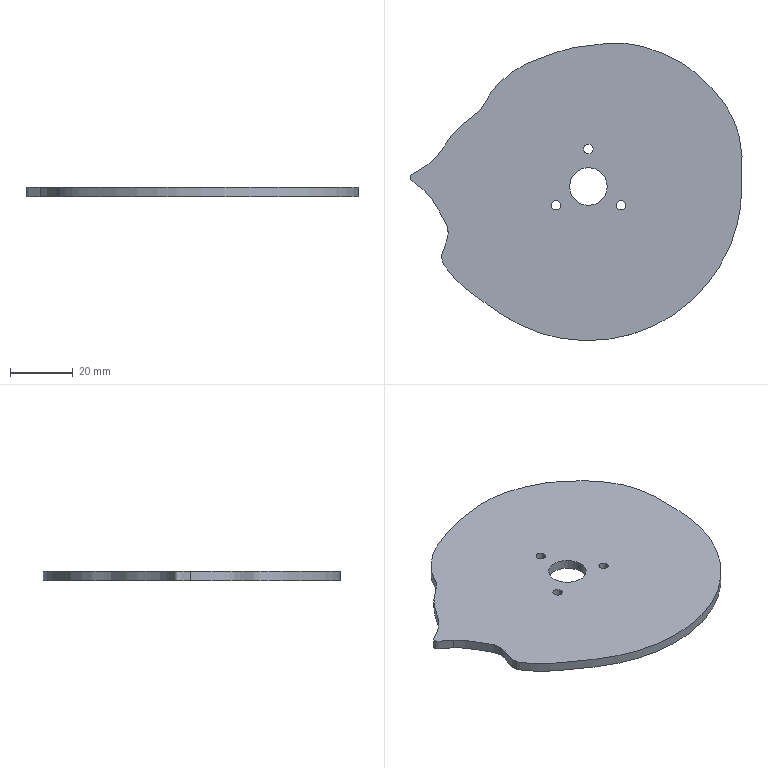Part | SolidWorks | features ICE 2, CurveInFile 1, Extrusion 1 | 1 solid | 12 faces | box 106.214 x 95.117 x 3 mm | volume 21730 mm3 | cylinder 8 | spline 2 | plane 2 | commonest cylinder face diameters 3 x6 12 x2